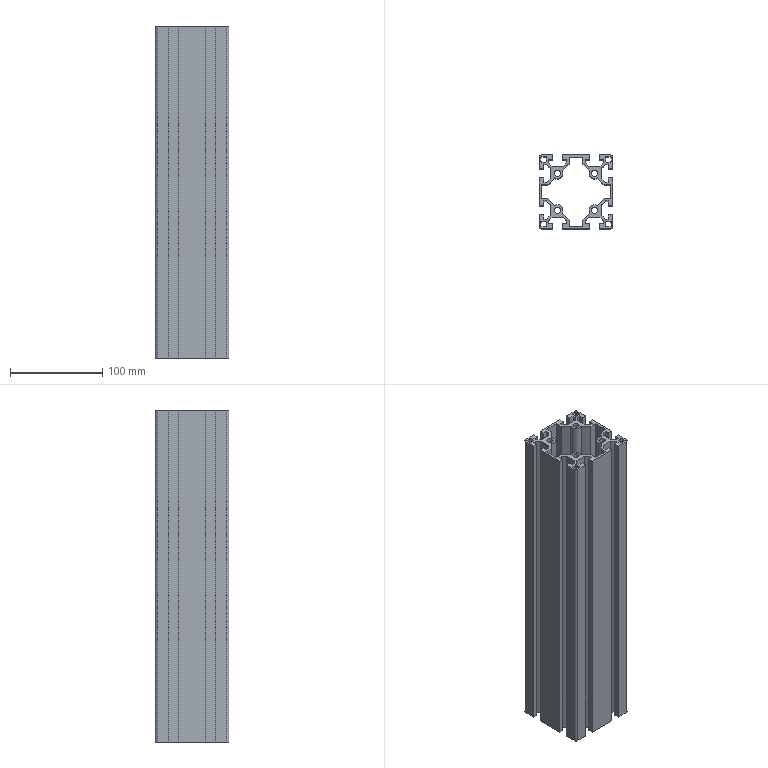Part | NX | 1 solid | 156 faces | box 80 x 80 x 360 mm | volume 630721 mm3 | plane 122 | cylinder 34 | commonest cylinder face diameters 2 x16 6.8 x8 11.8 x6 5.64 x4